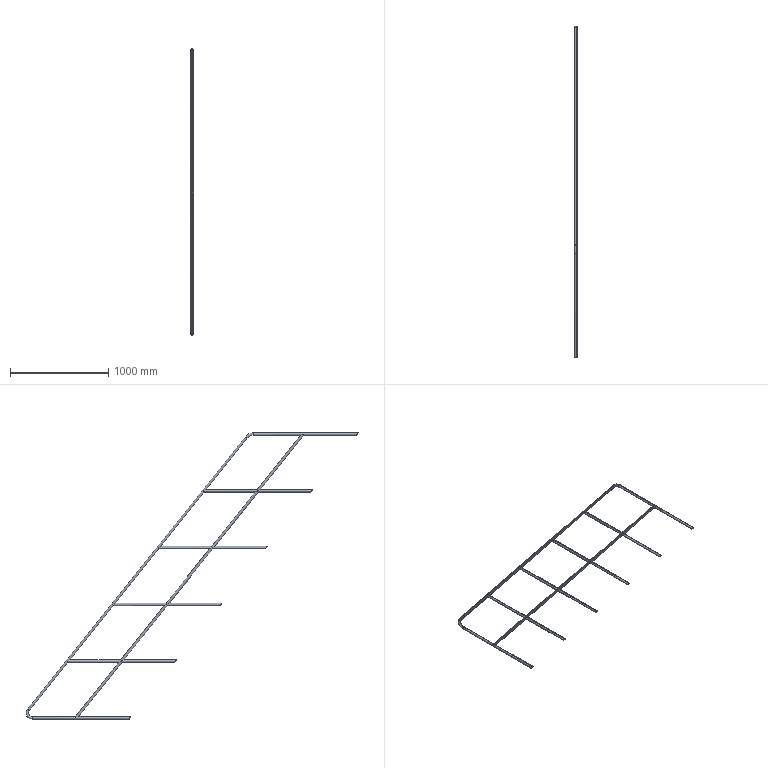Part | STEP file | 粉仓楼梯护栏1主体_Default<As Machined> | 14 solids | 94 faces | box 25 x 3380 x 2914 mm | volume 1521542 mm3 | cylinder 72 | plane 14 | torus 8 | commonest cylinder face diameters 25 x48 22 x24